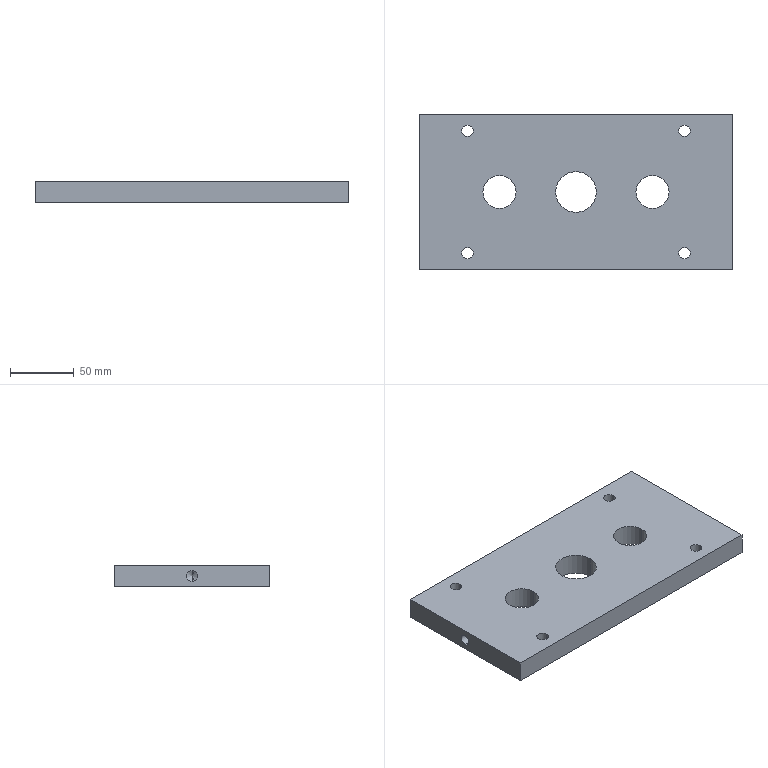Part | STEP file | 8 | 1 solid | 60 faces | box 246 x 122 x 17 mm | volume 467682 mm3 | cylinder 32 | cone 18 | plane 10 | commonest cylinder face diameters 4.134 x8 9 x8 15 x8 26 x4 8.5 x2 32 x2